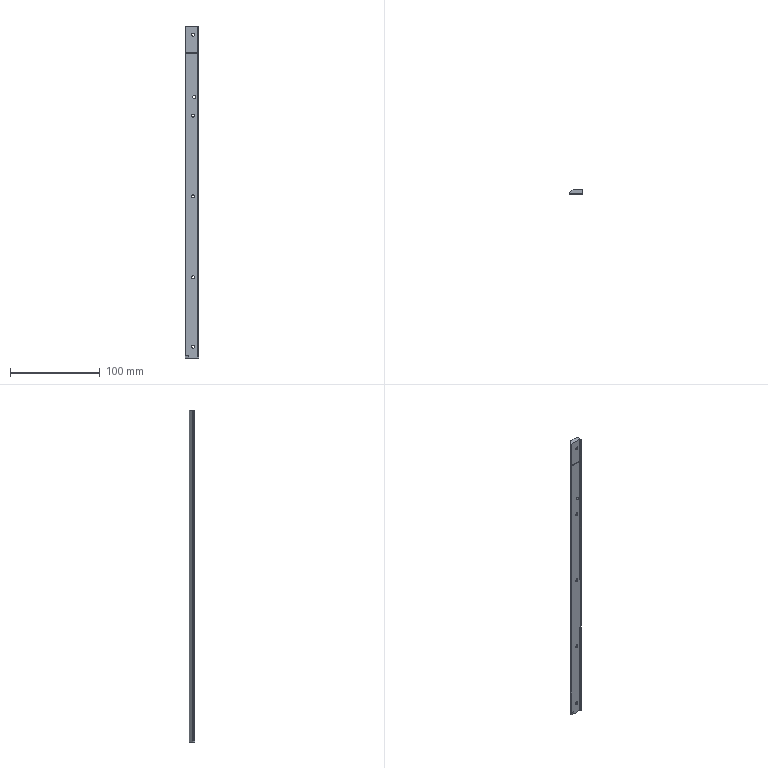Part | STEP file | 11-FG-B07611 | 1 solid | 45 faces | box 14.5 x 6 x 369.8 mm | volume 23525 mm3 | cylinder 23 | plane 22 | commonest cylinder face diameters 3.4 x10 6.5 x10 3.3 x2 0.85 x1
STEP:
#1=CARTESIAN_POINT('',(9.5,0.,289.15));
#2=VERTEX_POINT('',#1);
#3=CARTESIAN_POINT('',(9.5,0.,292.45));
#4=VERTEX_POINT('',#3);
#5=CARTESIAN_POINT('',(9.5,0.,290.8));
#6=DIRECTION('',(0.,1.,0.));
#7=DIRECTION('',(0.,0.,1.));
#8=AXIS2_PLACEMENT_3D('',#5,#6,#7);
#9=CIRCLE('',#8,1.65);
#10=EDGE_CURVE('',#2,#4,#9,.T.);
#11=ORIENTED_EDGE('',*,*,#10,.F.);
#12=CARTESIAN_POINT('',(9.5,5.,289.15));
#13=VERTEX_POINT('',#12);
#14=CARTESIAN_POINT('',(9.5,5.,289.15));
#15=DIRECTION('',(0.,1.,0.));
#16=VECTOR('',#15,1000.);
#17=LINE('',#14,#16);
#18=EDGE_CURVE('',#2,#13,#17,.T.);
#19=ORIENTED_EDGE('',*,*,#18,.T.);
#20=CARTESIAN_POINT('',(9.5,5.,292.45));
#21=VERTEX_POINT('',#20);
#22=CARTESIAN_POINT('',(9.5,5.,290.8));
#23=DIRECTION('',(0.,1.,0.));
#24=DIRECTION('',(0.,0.,1.));
#25=AXIS2_PLACEMENT_3D('',#22,#23,#24);
#26=CIRCLE('',#25,1.65);
#27=EDGE_CURVE('',#13,#21,#26,.T.);
#28=ORIENTED_EDGE('',*,*,#27,.T.);
#29=CARTESIAN_POINT('',(9.5,5.,292.45));
#30=DIRECTION('',(0.,1.,0.));
#31=VECTOR('',#30,1000.);
#32=LINE('',#29,#31);
#33=EDGE_CURVE('',#4,#21,#32,.T.);
#34=ORIENTED_EDGE('',*,*,#33,.F.);
#35=EDGE_LOOP('',(#11,#19,#28,#34));
#36=FACE_OUTER_BOUND('',#35,.T.);
#37=CARTESIAN_POINT('',(9.5,5.,290.8));
#38=DIRECTION('',(0.,1.,0.));
#39=DIRECTION('',(0.,0.,1.));
#40=AXIS2_PLACEMENT_3D('',#37,#38,#39);
#41=CYLINDRICAL_SURFACE('',#40,1.65);
#42=ADVANCED_FACE('',(#36),#41,.F.);
#43=CARTESIAN_POINT('',(8.5,1.6,356.75));
#44=VERTEX_POINT('',#43);
#45=CARTESIAN_POINT('',(8.5,1.6,363.25));
#46=VERTEX_POINT('',#45);
#47=CARTESIAN_POINT('',(8.5,1.6,360.));
#48=DIRECTION('',(0.,1.,0.));
#49=DIRECTION('',(0.,0.,1.));
#50=AXIS2_PLACEMENT_3D('',#47,#48,#49);
#51=CIRCLE('',#50,3.25);
#52=EDGE_CURVE('',#44,#46,#51,.T.);
#53=ORIENTED_EDGE('',*,*,#52,.F.);
#54=CARTESIAN_POINT('',(8.5,5.,356.75));
#55=VERTEX_POINT('',#54);
#56=CARTESIAN_POINT('',(8.5,5.,356.75));
#57=DIRECTION('',(0.,1.,0.));
#58=VECTOR('',#57,1000.);
#59=LINE('',#56,#58);
#60=EDGE_CURVE('',#44,#55,#59,.T.);
#61=ORIENTED_EDGE('',*,*,#60,.T.);
#62=CARTESIAN_POINT('',(8.5,5.,363.25));
#63=VERTEX_POINT('',#62);
#64=CARTESIAN_POINT('',(8.5,5.,360.));
#65=DIRECTION('',(0.,1.,0.));
#66=DIRECTION('',(0.,0.,1.));
#67=AXIS2_PLACEMENT_3D('',#64,#65,#66);
#68=CIRCLE('',#67,3.25);
#69=EDGE_CURVE('',#55,#63,#68,.T.);
#70=ORIENTED_EDGE('',*,*,#69,.T.);
#71=CARTESIAN_POINT('',(8.5,5.,363.25));
#72=DIRECTION('',(0.,1.,0.));
#73=VECTOR('',#72,1000.);
#74=LINE('',#71,#73);
#75=EDGE_CURVE('',#46,#63,#74,.T.);
#76=ORIENTED_EDGE('',*,*,#75,.F.);
#77=EDGE_LOOP('',(#53,#61,#70,#76));
#78=FACE_OUTER_BOUND('',#77,.T.);
#79=CARTESIAN_POINT('',(8.5,5.,360.));
#80=DIRECTION('',(0.,1.,0.));
#81=DIRECTION('',(0.,0.,1.));
#82=AXIS2_PLACEMENT_3D('',#79,#80,#81);
#83=CYLINDRICAL_SURFACE('',#82,3.25);
#84=ADVANCED_FACE('',(#78),#83,.F.);
#85=CARTESIAN_POINT('',(8.5,0.,358.3));
#86=VERTEX_POINT('',#85);
#87=CARTESIAN_POINT('',(8.5,0.,361.7));
#88=VERTEX_POINT('',#87);
#89=CARTESIAN_POINT('',(8.5,0.,360.));
#90=DIRECTION('',(0.,1.,0.));
#91=DIRECTION('',(0.,0.,1.));
#92=AXIS2_PLACEMENT_3D('',#89,#90,#91);
#93=CIRCLE('',#92,1.7);
#94=EDGE_CURVE('',#86,#88,#93,.T.);
#95=ORIENTED_EDGE('',*,*,#94,.F.);
#96=CARTESIAN_POINT('',(8.5,1.6,358.3));
#97=VERTEX_POINT('',#96);
#98=CARTESIAN_POINT('',(8.5,5.,358.3));
#99=DIRECTION('',(0.,1.,0.));
#100=VECTOR('',#99,1000.);
#101=LINE('',#98,#100);
#102=EDGE_CURVE('',#86,#97,#101,.T.);
#103=ORIENTED_EDGE('',*,*,#102,.T.);
#104=CARTESIAN_POINT('',(8.5,1.6,361.7));
#105=VERTEX_POINT('',#104);
#106=CARTESIAN_POINT('',(8.5,1.6,360.));
#107=DIRECTION('',(0.,1.,0.));
#108=DIRECTION('',(0.,0.,1.));
#109=AXIS2_PLACEMENT_3D('',#106,#107,#108);
#110=CIRCLE('',#109,1.7);
#111=EDGE_CURVE('',#97,#105,#110,.T.);
#112=ORIENTED_EDGE('',*,*,#111,.T.);
#113=CARTESIAN_POINT('',(8.5,5.,361.7));
#114=DIRECTION('',(0.,1.,0.));
#115=VECTOR('',#114,1000.);
#116=LINE('',#113,#115);
#117=EDGE_CURVE('',#88,#105,#116,.T.);
#118=ORIENTED_EDGE('',*,*,#117,.F.);
#119=EDGE_LOOP('',(#95,#103,#112,#118));
#120=FACE_OUTER_BOUND('',#119,.T.);
#121=CARTESIAN_POINT('',(8.5,5.,360.));
#122=DIRECTION('',(0.,1.,0.));
#123=DIRECTION('',(0.,0.,1.));
#124=AXIS2_PLACEMENT_3D('',#121,#122,#123);
#125=CYLINDRICAL_SURFACE('',#124,1.7);
#126=ADVANCED_FACE('',(#120),#125,.F.);
#127=CARTESIAN_POINT('',(8.5,1.6,266.75));
#128=VERTEX_POINT('',#127);
#129=CARTESIAN_POINT('',(8.5,1.6,273.25));
#130=VERTEX_POINT('',#129);
#131=CARTESIAN_POINT('',(8.5,1.6,270.));
#132=DIRECTION('',(0.,1.,0.));
#133=DIRECTION('',(0.,0.,1.));
#134=AXIS2_PLACEMENT_3D('',#131,#132,#133);
#135=CIRCLE('',#134,3.25);
#136=EDGE_CURVE('',#128,#130,#135,.T.);
#137=ORIENTED_EDGE('',*,*,#136,.F.);
#138=CARTESIAN_POINT('',(8.5,5.,266.75));
#139=VERTEX_POINT('',#138);
#140=CARTESIAN_POINT('',(8.5,5.,266.75));
#141=DIRECTION('',(0.,1.,0.));
#142=VECTOR('',#141,1000.);
#143=LINE('',#140,#142);
#144=EDGE_CURVE('',#128,#139,#143,.T.);
#145=ORIENTED_EDGE('',*,*,#144,.T.);
#146=CARTESIAN_POINT('',(8.5,5.,273.25));
#147=VERTEX_POINT('',#146);
#148=CARTESIAN_POINT('',(8.5,5.,270.));
#149=DIRECTION('',(0.,1.,0.));
#150=DIRECTION('',(0.,0.,1.));
#151=AXIS2_PLACEMENT_3D('',#148,#149,#150);
#152=CIRCLE('',#151,3.25);
#153=EDGE_CURVE('',#139,#147,#152,.T.);
#154=ORIENTED_EDGE('',*,*,#153,.T.);
#155=CARTESIAN_POINT('',(8.5,5.,273.25));
#156=DIRECTION('',(0.,1.,0.));
#157=VECTOR('',#156,1000.);
#158=LINE('',#155,#157);
#159=EDGE_CURVE('',#130,#147,#158,.T.);
#160=ORIENTED_EDGE('',*,*,#159,.F.);
#161=EDGE_LOOP('',(#137,#145,#154,#160));
#162=FACE_OUTER_BOUND('',#161,.T.);
#163=CARTESIAN_POINT('',(8.5,5.,270.));
#164=DIRECTION('',(0.,1.,0.));
#165=DIRECTION('',(0.,0.,1.));
#166=AXIS2_PLACEMENT_3D('',#163,#164,#165);
#167=CYLINDRICAL_SURFACE('',#166,3.25);
#168=ADVANCED_FACE('',(#162),#167,.F.);
#169=CARTESIAN_POINT('',(8.5,0.,268.3));
#170=VERTEX_POINT('',#169);
#171=CARTESIAN_POINT('',(8.5,0.,271.7));
#172=VERTEX_POINT('',#171);
#173=CARTESIAN_POINT('',(8.5,0.,270.));
#174=DIRECTION('',(0.,1.,0.));
#175=DIRECTION('',(0.,0.,1.));
#176=AXIS2_PLACEMENT_3D('',#173,#174,#175);
#177=CIRCLE('',#176,1.7);
#178=EDGE_CURVE('',#170,#172,#177,.T.);
#179=ORIENTED_EDGE('',*,*,#178,.F.);
#180=CARTESIAN_POINT('',(8.5,1.6,268.3));
#181=VERTEX_POINT('',#180);
#182=CARTESIAN_POINT('',(8.5,5.,268.3));
#183=DIRECTION('',(0.,1.,0.));
#184=VECTOR('',#183,1000.);
#185=LINE('',#182,#184);
#186=EDGE_CURVE('',#170,#181,#185,.T.);
#187=ORIENTED_EDGE('',*,*,#186,.T.);
#188=CARTESIAN_POINT('',(8.5,1.6,271.7));
#189=VERTEX_POINT('',#188);
#190=CARTESIAN_POINT('',(8.5,1.6,270.));
#191=DIRECTION('',(0.,1.,0.));
#192=DIRECTION('',(0.,0.,1.));
#193=AXIS2_PLACEMENT_3D('',#190,#191,#192);
#194=CIRCLE('',#193,1.7);
#195=EDGE_CURVE('',#181,#189,#194,.T.);
#196=ORIENTED_EDGE('',*,*,#195,.T.);
#197=CARTESIAN_POINT('',(8.5,5.,271.7));
#198=DIRECTION('',(0.,1.,0.));
#199=VECTOR('',#198,1000.);
#200=LINE('',#197,#199);
#201=EDGE_CURVE('',#172,#189,#200,.T.);
#202=ORIENTED_EDGE('',*,*,#201,.F.);
#203=EDGE_LOOP('',(#179,#187,#196,#202));
#204=FACE_OUTER_BOUND('',#203,.T.);
#205=CARTESIAN_POINT('',(8.5,5.,270.));
#206=DIRECTION('',(0.,1.,0.));
#207=DIRECTION('',(0.,0.,1.));
#208=AXIS2_PLACEMENT_3D('',#205,#206,#207);
#209=CYLINDRICAL_SURFACE('',#208,1.7);
#210=ADVANCED_FACE('',(#204),#209,.F.);
#211=CARTESIAN_POINT('',(8.5,1.6,176.75));
#212=VERTEX_POINT('',#211);
#213=CARTESIAN_POINT('',(8.5,1.6,183.25));
#214=VERTEX_POINT('',#213);
#215=CARTESIAN_POINT('',(8.5,1.6,180.));
#216=DIRECTION('',(0.,1.,0.));
#217=DIRECTION('',(0.,0.,1.));
#218=AXIS2_PLACEMENT_3D('',#215,#216,#217);
#219=CIRCLE('',#218,3.25);
#220=EDGE_CURVE('',#212,#214,#219,.T.);
#221=ORIENTED_EDGE('',*,*,#220,.F.);
#222=CARTESIAN_POINT('',(8.5,5.,176.75));
#223=VERTEX_POINT('',#222);
#224=CARTESIAN_POINT('',(8.5,5.,176.75));
#225=DIRECTION('',(0.,1.,0.));
#226=VECTOR('',#225,1000.);
#227=LINE('',#224,#226);
#228=EDGE_CURVE('',#212,#223,#227,.T.);
#229=ORIENTED_EDGE('',*,*,#228,.T.);
#230=CARTESIAN_POINT('',(8.5,5.,183.25));
#231=VERTEX_POINT('',#230);
#232=CARTESIAN_POINT('',(8.5,5.,180.));
#233=DIRECTION('',(0.,1.,0.));
#234=DIRECTION('',(0.,0.,1.));
#235=AXIS2_PLACEMENT_3D('',#232,#233,#234);
#236=CIRCLE('',#235,3.25);
#237=EDGE_CURVE('',#223,#231,#236,.T.);
#238=ORIENTED_EDGE('',*,*,#237,.T.);
#239=CARTESIAN_POINT('',(8.5,5.,183.25));
#240=DIRECTION('',(0.,1.,0.));
#241=VECTOR('',#240,1000.);
#242=LINE('',#239,#241);
#243=EDGE_CURVE('',#214,#231,#242,.T.);
#244=ORIENTED_EDGE('',*,*,#243,.F.);
#245=EDGE_LOOP('',(#221,#229,#238,#244));
#246=FACE_OUTER_BOUND('',#245,.T.);
#247=CARTESIAN_POINT('',(8.5,5.,180.));
#248=DIRECTION('',(0.,1.,0.));
#249=DIRECTION('',(0.,0.,1.));
#250=AXIS2_PLACEMENT_3D('',#247,#248,#249);
#251=CYLINDRICAL_SURFACE('',#250,3.25);
#252=ADVANCED_FACE('',(#246),#251,.F.);
#253=CARTESIAN_POINT('',(8.5,0.,178.3));
#254=VERTEX_POINT('',#253);
#255=CARTESIAN_POINT('',(8.5,0.,181.7));
#256=VERTEX_POINT('',#255);
#257=CARTESIAN_POINT('',(8.5,0.,180.));
#258=DIRECTION('',(0.,1.,0.));
#259=DIRECTION('',(0.,0.,1.));
#260=AXIS2_PLACEMENT_3D('',#257,#258,#259);
#261=CIRCLE('',#260,1.7);
#262=EDGE_CURVE('',#254,#256,#261,.T.);
#263=ORIENTED_EDGE('',*,*,#262,.F.);
#264=CARTESIAN_POINT('',(8.5,1.6,178.3));
#265=VERTEX_POINT('',#264);
#266=CARTESIAN_POINT('',(8.5,5.,178.3));
#267=DIRECTION('',(0.,1.,0.));
#268=VECTOR('',#267,1000.);
#269=LINE('',#266,#268);
#270=EDGE_CURVE('',#254,#265,#269,.T.);
#271=ORIENTED_EDGE('',*,*,#270,.T.);
#272=CARTESIAN_POINT('',(8.5,1.6,181.7));
#273=VERTEX_POINT('',#272);
#274=CARTESIAN_POINT('',(8.5,1.6,180.));
#275=DIRECTION('',(0.,1.,0.));
#276=DIRECTION('',(0.,0.,1.));
#277=AXIS2_PLACEMENT_3D('',#274,#275,#276);
#278=CIRCLE('',#277,1.7);
#279=EDGE_CURVE('',#265,#273,#278,.T.);
#280=ORIENTED_EDGE('',*,*,#279,.T.);
#281=CARTESIAN_POINT('',(8.5,5.,181.7));
#282=DIRECTION('',(0.,1.,0.));
#283=VECTOR('',#282,1000.);
#284=LINE('',#281,#283);
#285=EDGE_CURVE('',#256,#273,#284,.T.);
#286=ORIENTED_EDGE('',*,*,#285,.F.);
#287=EDGE_LOOP('',(#263,#271,#280,#286));
#288=FACE_OUTER_BOUND('',#287,.T.);
#289=CARTESIAN_POINT('',(8.5,5.,180.));
#290=DIRECTION('',(0.,1.,0.));
#291=DIRECTION('',(0.,0.,1.));
#292=AXIS2_PLACEMENT_3D('',#289,#290,#291);
#293=CYLINDRICAL_SURFACE('',#292,1.7);
#294=ADVANCED_FACE('',(#288),#293,.F.);
#295=CARTESIAN_POINT('',(8.5,1.6,86.75));
#296=VERTEX_POINT('',#295);
#297=CARTESIAN_POINT('',(8.5,1.6,93.25));
#298=VERTEX_POINT('',#297);
#299=CARTESIAN_POINT('',(8.5,1.6,90.));
#300=DIRECTION('',(0.,1.,0.));
#301=DIRECTION('',(0.,0.,1.));
#302=AXIS2_PLACEMENT_3D('',#299,#300,#301);
#303=CIRCLE('',#302,3.25);
#304=EDGE_CURVE('',#296,#298,#303,.T.);
#305=ORIENTED_EDGE('',*,*,#304,.F.);
#306=CARTESIAN_POINT('',(8.5,5.,86.75));
#307=VERTEX_POINT('',#306);
#308=CARTESIAN_POINT('',(8.5,5.,86.75));
#309=DIRECTION('',(0.,1.,0.));
#310=VECTOR('',#309,1000.);
#311=LINE('',#308,#310);
#312=EDGE_CURVE('',#296,#307,#311,.T.);
#313=ORIENTED_EDGE('',*,*,#312,.T.);
#314=CARTESIAN_POINT('',(8.5,5.,93.25));
#315=VERTEX_POINT('',#314);
#316=CARTESIAN_POINT('',(8.5,5.,90.));
#317=DIRECTION('',(0.,1.,0.));
#318=DIRECTION('',(0.,0.,1.));
#319=AXIS2_PLACEMENT_3D('',#316,#317,#318);
#320=CIRCLE('',#319,3.25);
#321=EDGE_CURVE('',#307,#315,#320,.T.);
#322=ORIENTED_EDGE('',*,*,#321,.T.);
#323=CARTESIAN_POINT('',(8.5,5.,93.25));
#324=DIRECTION('',(0.,1.,0.));
#325=VECTOR('',#324,1000.);
#326=LINE('',#323,#325);
#327=EDGE_CURVE('',#298,#315,#326,.T.);
#328=ORIENTED_EDGE('',*,*,#327,.F.);
#329=EDGE_LOOP('',(#305,#313,#322,#328));
#330=FACE_OUTER_BOUND('',#329,.T.);
#331=CARTESIAN_POINT('',(8.5,5.,90.));
#332=DIRECTION('',(0.,1.,0.));
#333=DIRECTION('',(0.,0.,1.));
#334=AXIS2_PLACEMENT_3D('',#331,#332,#333);
#335=CYLINDRICAL_SURFACE('',#334,3.25);
#336=ADVANCED_FACE('',(#330),#335,.F.);
#337=CARTESIAN_POINT('',(8.5,0.,88.3));
#338=VERTEX_POINT('',#337);
#339=CARTESIAN_POINT('',(8.5,0.,91.7));
#340=VERTEX_POINT('',#339);
#341=CARTESIAN_POINT('',(8.5,0.,90.));
#342=DIRECTION('',(0.,1.,0.));
#343=DIRECTION('',(0.,0.,1.));
#344=AXIS2_PLACEMENT_3D('',#341,#342,#343);
#345=CIRCLE('',#344,1.7);
#346=EDGE_CURVE('',#338,#340,#345,.T.);
#347=ORIENTED_EDGE('',*,*,#346,.F.);
#348=CARTESIAN_POINT('',(8.5,1.6,88.3));
#349=VERTEX_POINT('',#348);
#350=CARTESIAN_POINT('',(8.5,5.,88.3));
#351=DIRECTION('',(0.,1.,0.));
#352=VECTOR('',#351,1000.);
#353=LINE('',#350,#352);
#354=EDGE_CURVE('',#338,#349,#353,.T.);
#355=ORIENTED_EDGE('',*,*,#354,.T.);
#356=CARTESIAN_POINT('',(8.5,1.6,91.7));
#357=VERTEX_POINT('',#356);
#358=CARTESIAN_POINT('',(8.5,1.6,90.));
#359=DIRECTION('',(0.,1.,0.));
#360=DIRECTION('',(0.,0.,1.));
#361=AXIS2_PLACEMENT_3D('',#358,#359,#360);
#362=CIRCLE('',#361,1.7);
#363=EDGE_CURVE('',#349,#357,#362,.T.);
#364=ORIENTED_EDGE('',*,*,#363,.T.);
#365=CARTESIAN_POINT('',(8.5,5.,91.7));
#366=DIRECTION('',(0.,1.,0.));
#367=VECTOR('',#366,1000.);
#368=LINE('',#365,#367);
#369=EDGE_CURVE('',#340,#357,#368,.T.);
#370=ORIENTED_EDGE('',*,*,#369,.F.);
#371=EDGE_LOOP('',(#347,#355,#364,#370));
#372=FACE_OUTER_BOUND('',#371,.T.);
#373=CARTESIAN_POINT('',(8.5,5.,90.));
#374=DIRECTION('',(0.,1.,0.));
#375=DIRECTION('',(0.,0.,1.));
#376=AXIS2_PLACEMENT_3D('',#373,#374,#375);
#377=CYLINDRICAL_SURFACE('',#376,1.7);
#378=ADVANCED_FACE('',(#372),#377,.F.);
#379=CARTESIAN_POINT('',(8.5,1.6,9.25));
#380=VERTEX_POINT('',#379);
#381=CARTESIAN_POINT('',(8.5,1.6,15.75));
#382=VERTEX_POINT('',#381);
#383=CARTESIAN_POINT('',(8.5,1.6,12.5));
#384=DIRECTION('',(0.,1.,0.));
#385=DIRECTION('',(0.,0.,1.));
#386=AXIS2_PLACEMENT_3D('',#383,#384,#385);
#387=CIRCLE('',#386,3.25);
#388=EDGE_CURVE('',#380,#382,#387,.T.);
#389=ORIENTED_EDGE('',*,*,#388,.F.);
#390=CARTESIAN_POINT('',(8.5,5.,9.25));
#391=VERTEX_POINT('',#390);
#392=CARTESIAN_POINT('',(8.5,5.,9.25));
#393=DIRECTION('',(0.,1.,0.));
#394=VECTOR('',#393,1000.);
#395=LINE('',#392,#394);
#396=EDGE_CURVE('',#380,#391,#395,.T.);
#397=ORIENTED_EDGE('',*,*,#396,.T.);
#398=CARTESIAN_POINT('',(8.5,5.,15.75));
#399=VERTEX_POINT('',#398);
#400=CARTESIAN_POINT('',(8.5,5.,12.5));
#401=DIRECTION('',(0.,1.,0.));
#402=DIRECTION('',(0.,0.,1.));
#403=AXIS2_PLACEMENT_3D('',#400,#401,#402);
#404=CIRCLE('',#403,3.25);
#405=EDGE_CURVE('',#391,#399,#404,.T.);
#406=ORIENTED_EDGE('',*,*,#405,.T.);
#407=CARTESIAN_POINT('',(8.5,5.,15.75));
#408=DIRECTION('',(0.,1.,0.));
#409=VECTOR('',#408,1000.);
#410=LINE('',#407,#409);
#411=EDGE_CURVE('',#382,#399,#410,.T.);
#412=ORIENTED_EDGE('',*,*,#411,.F.);
#413=EDGE_LOOP('',(#389,#397,#406,#412));
#414=FACE_OUTER_BOUND('',#413,.T.);
#415=CARTESIAN_POINT('',(8.5,5.,12.5));
#416=DIRECTION('',(0.,1.,0.));
#417=DIRECTION('',(0.,0.,1.));
#418=AXIS2_PLACEMENT_3D('',#415,#416,#417);
#419=CYLINDRICAL_SURFACE('',#418,3.25);
#420=ADVANCED_FACE('',(#414),#419,.F.);
#421=CARTESIAN_POINT('',(8.5,0.,10.8));
#422=VERTEX_POINT('',#421);
#423=CARTESIAN_POINT('',(8.5,0.,14.2));
#424=VERTEX_POINT('',#423);
#425=CARTESIAN_POINT('',(8.5,0.,12.5));
#426=DIRECTION('',(0.,1.,0.));
#427=DIRECTION('',(0.,0.,1.));
#428=AXIS2_PLACEMENT_3D('',#425,#426,#427);
#429=CIRCLE('',#428,1.7);
#430=EDGE_CURVE('',#422,#424,#429,.T.);
#431=ORIENTED_EDGE('',*,*,#430,.F.);
#432=CARTESIAN_POINT('',(8.5,1.6,10.8));
#433=VERTEX_POINT('',#432);
#434=CARTESIAN_POINT('',(8.5,5.,10.8));
#435=DIRECTION('',(0.,1.,0.));
#436=VECTOR('',#435,1000.);
#437=LINE('',#434,#436);
#438=EDGE_CURVE('',#422,#433,#437,.T.);
#439=ORIENTED_EDGE('',*,*,#438,.T.);
#440=CARTESIAN_POINT('',(8.5,1.6,14.2));
#441=VERTEX_POINT('',#440);
#442=CARTESIAN_POINT('',(8.5,1.6,12.5));
#443=DIRECTION('',(0.,1.,0.));
#444=DIRECTION('',(0.,0.,1.));
#445=AXIS2_PLACEMENT_3D('',#442,#443,#444);
#446=CIRCLE('',#445,1.7);
#447=EDGE_CURVE('',#433,#441,#446,.T.);
#448=ORIENTED_EDGE('',*,*,#447,.T.);
#449=CARTESIAN_POINT('',(8.5,5.,14.2));
#450=DIRECTION('',(0.,1.,0.));
#451=VECTOR('',#450,1000.);
#452=LINE('',#449,#451);
#453=EDGE_CURVE('',#424,#441,#452,.T.);
#454=ORIENTED_EDGE('',*,*,#453,.F.);
#455=EDGE_LOOP('',(#431,#439,#448,#454));
#456=FACE_OUTER_BOUND('',#455,.T.);
#457=CARTESIAN_POINT('',(8.5,5.,12.5));
#458=DIRECTION('',(0.,1.,0.));
#459=DIRECTION('',(0.,0.,1.));
#460=AXIS2_PLACEMENT_3D('',#457,#458,#459);
#461=CYLINDRICAL_SURFACE('',#460,1.7);
#462=ADVANCED_FACE('',(#456),#461,.F.);
#463=CARTESIAN_POINT('',(0.,0.,369.8));
#464=VERTEX_POINT('',#463);
#465=CARTESIAN_POINT('',(0.,0.,340.425));
#466=VERTEX_POINT('',#465);
#467=CARTESIAN_POINT('',(0.,0.,370.));
#468=DIRECTION('',(0.,0.,-1.));
#469=VECTOR('',#468,1000.);
#470=LINE('',#467,#469);
#471=EDGE_CURVE('',#464,#466,#470,.T.);
#472=ORIENTED_EDGE('',*,*,#471,.F.);
#473=CARTESIAN_POINT('',(0.,1.,369.8));
#474=VERTEX_POINT('',#473);
#475=CARTESIAN_POINT('',(0.,-42.,369.8));
#476=DIRECTION('',(0.,1.,0.));
#477=VECTOR('',#476,1000.);
#478=LINE('',#475,#477);
#479=EDGE_CURVE('',#464,#474,#478,.T.);
#480=ORIENTED_EDGE('',*,*,#479,.T.);
#481=CARTESIAN_POINT('',(0.,1.,340.144));
#482=VERTEX_POINT('',#481);
#483=CARTESIAN_POINT('',(0.,1.,370.));
#484=DIRECTION('',(0.,0.,-1.));
#485=VECTOR('',#484,1000.);
#486=LINE('',#483,#485);
#487=EDGE_CURVE('',#474,#482,#486,.T.);
#488=ORIENTED_EDGE('',*,*,#487,.T.);
#489=CARTESIAN_POINT('',(0.,0.6,340.425));
#490=VERTEX_POINT('',#489);
#491=CARTESIAN_POINT('',(0.,0.6,340.));
#492=DIRECTION('',(-1.,0.,0.));
#493=DIRECTION('',(0.,0.,1.));
#494=AXIS2_PLACEMENT_3D('',#491,#492,#493);
#495=CIRCLE('',#494,0.425);
#496=EDGE_CURVE('',#490,#482,#495,.T.);
#497=ORIENTED_EDGE('',*,*,#496,.F.);
#498=CARTESIAN_POINT('',(0.,0.6,340.425));
#499=DIRECTION('',(0.,1.,0.));
#500=VECTOR('',#499,1000.);
#501=LINE('',#498,#500);
#502=EDGE_CURVE('',#466,#490,#501,.T.);
#503=ORIENTED_EDGE('',*,*,#502,.F.);
#504=EDGE_LOOP('',(#472,#480,#488,#497,#503));
#505=FACE_OUTER_BOUND('',#504,.T.);
#506=CARTESIAN_POINT('',(0.,0.,370.));
#507=DIRECTION('',(1.,0.,0.));
#508=DIRECTION('',(0.,1.,0.));
#509=AXIS2_PLACEMENT_3D('',#506,#507,#508);
#510=PLANE('',#509);
#511=ADVANCED_FACE('',(#505),#510,.F.);
#512=CARTESIAN_POINT('',(8.5,0.,360.));
#513=DIRECTION('',(0.,1.,0.));
#514=DIRECTION('',(0.,0.,1.));
#515=AXIS2_PLACEMENT_3D('',#512,#513,#514);
#516=CIRCLE('',#515,1.7);
#517=EDGE_CURVE('',#88,#86,#516,.T.);
#518=ORIENTED_EDGE('',*,*,#517,.T.);
#519=ORIENTED_EDGE('',*,*,#94,.T.);
#520=EDGE_LOOP('',(#518,#519));
#521=FACE_BOUND('',#520,.T.);
#522=CARTESIAN_POINT('',(13.5,0.,369.8));
#523=VERTEX_POINT('',#522);
#524=CARTESIAN_POINT('',(13.5,0.,340.425));
#525=VERTEX_POINT('',#524);
#526=CARTESIAN_POINT('',(13.5,0.,370.));
#527=DIRECTION('',(0.,0.,-1.));
#528=VECTOR('',#527,1000.);
#529=LINE('',#526,#528);
#530=EDGE_CURVE('',#523,#525,#529,.T.);
#531=ORIENTED_EDGE('',*,*,#530,.F.);
#532=CARTESIAN_POINT('',(0.,0.,369.8));
#533=DIRECTION('',(-1.,0.,0.));
#534=VECTOR('',#533,1000.);
#535=LINE('',#532,#534);
#536=EDGE_CURVE('',#523,#464,#535,.T.);
#537=ORIENTED_EDGE('',*,*,#536,.T.);
#538=ORIENTED_EDGE('',*,*,#471,.T.);
#539=CARTESIAN_POINT('',(13.5,0.,340.425));
#540=DIRECTION('',(-1.,0.,0.));
#541=VECTOR('',#540,1000.);
#542=LINE('',#539,#541);
#543=EDGE_CURVE('',#525,#466,#542,.T.);
#544=ORIENTED_EDGE('',*,*,#543,.F.);
#545=EDGE_LOOP('',(#531,#537,#538,#544));
#546=FACE_OUTER_BOUND('',#545,.T.);
#547=CARTESIAN_POINT('',(0.,0.,370.));
#548=DIRECTION('',(0.,1.,0.));
#549=DIRECTION('',(0.,0.,1.));
#550=AXIS2_PLACEMENT_3D('',#547,#548,#549);
#551=PLANE('',#550);
#552=ADVANCED_FACE('',(#521,#546),#551,.F.);
#553=CARTESIAN_POINT('',(0.,1.,0.));
#554=VERTEX_POINT('',#553);
#555=CARTESIAN_POINT('',(0.,0.8038,0.));
#556=VERTEX_POINT('',#555);
#557=CARTESIAN_POINT('',(0.,0.,0.));
#558=DIRECTION('',(0.,-1.,0.));
#559=VECTOR('',#558,1000.);
#560=LINE('',#557,#559);
#561=EDGE_CURVE('',#554,#556,#560,.T.);
#562=ORIENTED_EDGE('',*,*,#561,.T.);
#563=CARTESIAN_POINT('',(0.,0.,3.));
#564=VERTEX_POINT('',#563);
#565=CARTESIAN_POINT('',(0.,0.,3.));
#566=DIRECTION('',(0.,0.2588,-0.9659));
#567=VECTOR('',#566,1000.);
#568=LINE('',#565,#567);
#569=EDGE_CURVE('',#564,#556,#568,.T.);
#570=ORIENTED_EDGE('',*,*,#569,.F.);
#571=CARTESIAN_POINT('',(0.,0.,339.575));
#572=VERTEX_POINT('',#571);
#573=CARTESIAN_POINT('',(0.,0.,370.));
#574=DIRECTION('',(0.,0.,-1.));
#575=VECTOR('',#574,1000.);
#576=LINE('',#573,#575);
#577=EDGE_CURVE('',#572,#564,#576,.T.);
#578=ORIENTED_EDGE('',*,*,#577,.F.);
#579=CARTESIAN_POINT('',(0.,0.6,339.575));
#580=VERTEX_POINT('',#579);
#581=CARTESIAN_POINT('',(0.,0.6,339.575));
#582=DIRECTION('',(0.,-1.,0.));
#583=VECTOR('',#582,1000.);
#584=LINE('',#581,#583);
#585=EDGE_CURVE('',#580,#572,#584,.T.);
#586=ORIENTED_EDGE('',*,*,#585,.F.);
#587=CARTESIAN_POINT('',(0.,1.,339.856));
#588=VERTEX_POINT('',#587);
#589=CARTESIAN_POINT('',(0.,0.6,340.));
#590=DIRECTION('',(-1.,0.,0.));
#591=DIRECTION('',(0.,0.,1.));
#592=AXIS2_PLACEMENT_3D('',#589,#590,#591);
#593=CIRCLE('',#592,0.425);
#594=EDGE_CURVE('',#588,#580,#593,.T.);
#595=ORIENTED_EDGE('',*,*,#594,.F.);
#596=CARTESIAN_POINT('',(0.,1.,370.));
#597=DIRECTION('',(0.,0.,-1.));
#598=VECTOR('',#597,1000.);
#599=LINE('',#596,#598);
#600=EDGE_CURVE('',#588,#554,#599,.T.);
#601=ORIENTED_EDGE('',*,*,#600,.T.);
#602=EDGE_LOOP('',(#562,#570,#578,#586,#595,#601));
#603=FACE_OUTER_BOUND('',#602,.T.);
#604=CARTESIAN_POINT('',(0.,0.,370.));
#605=DIRECTION('',(1.,0.,0.));
#606=DIRECTION('',(0.,1.,0.));
#607=AXIS2_PLACEMENT_3D('',#604,#605,#606);
#608=PLANE('',#607);
#609=ADVANCED_FACE('',(#603),#608,.F.);
#610=CARTESIAN_POINT('',(9.5,0.,290.8));
#611=DIRECTION('',(0.,1.,0.));
#612=DIRECTION('',(0.,0.,1.));
#613=AXIS2_PLACEMENT_3D('',#610,#611,#612);
#614=CIRCLE('',#613,1.65);
#615=EDGE_CURVE('',#4,#2,#614,.T.);
#616=ORIENTED_EDGE('',*,*,#615,.T.);
#617=ORIENTED_EDGE('',*,*,#10,.T.);
#618=EDGE_LOOP('',(#616,#617));
#619=FACE_BOUND('',#618,.T.);
#620=CARTESIAN_POINT('',(8.5,0.,270.));
#621=DIRECTION('',(0.,1.,0.));
#622=DIRECTION('',(0.,0.,1.));
#623=AXIS2_PLACEMENT_3D('',#620,#621,#622);
#624=CIRCLE('',#623,1.7);
#625=EDGE_CURVE('',#172,#170,#624,.T.);
#626=ORIENTED_EDGE('',*,*,#625,.T.);
#627=ORIENTED_EDGE('',*,*,#178,.T.);
#628=EDGE_LOOP('',(#626,#627));
#629=FACE_BOUND('',#628,.T.);
#630=CARTESIAN_POINT('',(8.5,0.,180.));
#631=DIRECTION('',(0.,1.,0.));
#632=DIRECTION('',(0.,0.,1.));
#633=AXIS2_PLACEMENT_3D('',#630,#631,#632);
#634=CIRCLE('',#633,1.7);
#635=EDGE_CURVE('',#256,#254,#634,.T.);
#636=ORIENTED_EDGE('',*,*,#635,.T.);
#637=ORIENTED_EDGE('',*,*,#262,.T.);
#638=EDGE_LOOP('',(#636,#637));
#639=FACE_BOUND('',#638,.T.);
#640=CARTESIAN_POINT('',(8.5,0.,90.));
#641=DIRECTION('',(0.,1.,0.));
#642=DIRECTION('',(0.,0.,1.));
#643=AXIS2_PLACEMENT_3D('',#640,#641,#642);
#644=CIRCLE('',#643,1.7);
#645=EDGE_CURVE('',#340,#338,#644,.T.);
#646=ORIENTED_EDGE('',*,*,#645,.T.);
#647=ORIENTED_EDGE('',*,*,#346,.T.);
#648=EDGE_LOOP('',(#646,#647));
#649=FACE_BOUND('',#648,.T.);
#650=CARTESIAN_POINT('',(8.5,0.,12.5));
#651=DIRECTION('',(0.,1.,0.));
#652=DIRECTION('',(0.,0.,1.));
#653=AXIS2_PLACEMENT_3D('',#650,#651,#652);
#654=CIRCLE('',#653,1.7);
#655=EDGE_CURVE('',#424,#422,#654,.T.);
#656=ORIENTED_EDGE('',*,*,#655,.T.);
#657=ORIENTED_EDGE('',*,*,#430,.T.);
#658=EDGE_LOOP('',(#656,#657));
#659=FACE_BOUND('',#658,.T.);
#660=CARTESIAN_POINT('',(3.5,0.,3.));
#661=VERTEX_POINT('',#660);
#662=CARTESIAN_POINT('',(3.5,0.,3.));
#663=DIRECTION('',(-1.,0.,0.));
#664=VECTOR('',#663,1000.);
#665=LINE('',#662,#664);
#666=EDGE_CURVE('',#661,#564,#665,.T.);
#667=ORIENTED_EDGE('',*,*,#666,.F.);
#668=CARTESIAN_POINT('',(4.304,0.,0.));
#669=VERTEX_POINT('',#668);
#670=CARTESIAN_POINT('',(3.5,0.,3.));
#671=DIRECTION('',(0.2588,0.,-0.9659));
#672=VECTOR('',#671,1000.);
#673=LINE('',#670,#672);
#674=EDGE_CURVE('',#661,#669,#673,.T.);
#675=ORIENTED_EDGE('',*,*,#674,.T.);
#676=CARTESIAN_POINT('',(13.5,0.,0.));
#677=VERTEX_POINT('',#676);
#678=CARTESIAN_POINT('',(0.,0.,0.));
#679=DIRECTION('',(1.,0.,0.));
#680=VECTOR('',#679,1000.);
#681=LINE('',#678,#680);
#682=EDGE_CURVE('',#669,#677,#681,.T.);
#683=ORIENTED_EDGE('',*,*,#682,.T.);
#684=CARTESIAN_POINT('',(13.5,0.,339.575));
#685=VERTEX_POINT('',#684);
#686=CARTESIAN_POINT('',(13.5,0.,370.));
#687=DIRECTION('',(0.,0.,-1.));
#688=VECTOR('',#687,1000.);
#689=LINE('',#686,#688);
#690=EDGE_CURVE('',#685,#677,#689,.T.);
#691=ORIENTED_EDGE('',*,*,#690,.F.);
#692=CARTESIAN_POINT('',(13.5,0.,339.575));
#693=DIRECTION('',(-1.,0.,0.));
#694=VECTOR('',#693,1000.);
#695=LINE('',#692,#694);
#696=EDGE_CURVE('',#685,#572,#695,.T.);
#697=ORIENTED_EDGE('',*,*,#696,.T.);
#698=ORIENTED_EDGE('',*,*,#577,.T.);
#699=EDGE_LOOP('',(#667,#675,#683,#691,#697,#698));
#700=FACE_OUTER_BOUND('',#699,.T.);
#701=CARTESIAN_POINT('',(0.,0.,370.));
#702=DIRECTION('',(0.,1.,0.));
#703=DIRECTION('',(0.,0.,1.));
#704=AXIS2_PLACEMENT_3D('',#701,#702,#703);
#705=PLANE('',#704);
#706=ADVANCED_FACE('',(#619,#629,#639,#649,#659,#700),#705,.F.);
#707=CARTESIAN_POINT('',(9.5,5.,290.8));
#708=DIRECTION('',(0.,1.,0.));
#709=DIRECTION('',(0.,0.,1.));
#710=AXIS2_PLACEMENT_3D('',#707,#708,#709);
#711=CIRCLE('',#710,1.65);
#712=EDGE_CURVE('',#21,#13,#711,.T.);
#713=ORIENTED_EDGE('',*,*,#712,.F.);
#714=ORIENTED_EDGE('',*,*,#27,.F.);
#715=EDGE_LOOP('',(#713,#714));
#716=FACE_BOUND('',#715,.T.);
#717=CARTESIAN_POINT('',(8.5,5.,360.));
#718=DIRECTION('',(0.,1.,0.));
#719=DIRECTION('',(0.,0.,1.));
#720=AXIS2_PLACEMENT_3D('',#717,#718,#719);
#721=CIRCLE('',#720,3.25);
#722=EDGE_CURVE('',#63,#55,#721,.T.);
#723=ORIENTED_EDGE('',*,*,#722,.F.);
#724=ORIENTED_EDGE('',*,*,#69,.F.);
#725=EDGE_LOOP('',(#723,#724));
#726=FACE_BOUND('',#725,.T.);
#727=CARTESIAN_POINT('',(8.5,5.,270.));
#728=DIRECTION('',(0.,1.,0.));
#729=DIRECTION('',(0.,0.,1.));
#730=AXIS2_PLACEMENT_3D('',#727,#728,#729);
#731=CIRCLE('',#730,3.25);
#732=EDGE_CURVE('',#147,#139,#731,.T.);
#733=ORIENTED_EDGE('',*,*,#732,.F.);
#734=ORIENTED_EDGE('',*,*,#153,.F.);
#735=EDGE_LOOP('',(#733,#734));
#736=FACE_BOUND('',#735,.T.);
#737=CARTESIAN_POINT('',(8.5,5.,180.));
#738=DIRECTION('',(0.,1.,0.));
#739=DIRECTION('',(0.,0.,1.));
#740=AXIS2_PLACEMENT_3D('',#737,#738,#739);
#741=CIRCLE('',#740,3.25);
#742=EDGE_CURVE('',#231,#223,#741,.T.);
#743=ORIENTED_EDGE('',*,*,#742,.F.);
#744=ORIENTED_EDGE('',*,*,#237,.F.);
#745=EDGE_LOOP('',(#743,#744));
#746=FACE_BOUND('',#745,.T.);
#747=CARTESIAN_POINT('',(8.5,5.,90.));
#748=DIRECTION('',(0.,1.,0.));
#749=DIRECTION('',(0.,0.,1.));
#750=AXIS2_PLACEMENT_3D('',#747,#748,#749);
#751=CIRCLE('',#750,3.25);
#752=EDGE_CURVE('',#315,#307,#751,.T.);
#753=ORIENTED_EDGE('',*,*,#752,.F.);
#754=ORIENTED_EDGE('',*,*,#321,.F.);
#755=EDGE_LOOP('',(#753,#754));
#756=FACE_BOUND('',#755,.T.);
#757=CARTESIAN_POINT('',(8.5,5.,12.5));
#758=DIRECTION('',(0.,1.,0.));
#759=DIRECTION('',(0.,0.,1.));
#760=AXIS2_PLACEMENT_3D('',#757,#758,#759);
#761=CIRCLE('',#760,3.25);
#762=EDGE_CURVE('',#399,#391,#761,.T.);
#763=ORIENTED_EDGE('',*,*,#762,.F.);
#764=ORIENTED_EDGE('',*,*,#405,.F.);
#765=EDGE_LOOP('',(#763,#764));
#766=FACE_BOUND('',#765,.T.);
#767=CARTESIAN_POINT('',(4.,5.,0.));
#768=VERTEX_POINT('',#767);
#769=CARTESIAN_POINT('',(4.,5.,369.8));
#770=VERTEX_POINT('',#769);
#771=CARTESIAN_POINT('',(4.,5.,370.));
#772=DIRECTION('',(0.,0.,1.));
#773=VECTOR('',#772,1000.);
#774=LINE('',#771,#773);
#775=EDGE_CURVE('',#768,#770,#774,.T.);
#776=ORIENTED_EDGE('',*,*,#775,.T.);
#777=CARTESIAN_POINT('',(14.5,5.,369.8));
#778=VERTEX_POINT('',#777);
#779=CARTESIAN_POINT('',(14.5,5.,369.8));
#780=DIRECTION('',(-1.,0.,0.));
#781=VECTOR('',#780,1000.);
#782=LINE('',#779,#781);
#783=EDGE_CURVE('',#778,#770,#782,.T.);
#784=ORIENTED_EDGE('',*,*,#783,.F.);
#785=CARTESIAN_POINT('',(14.5,5.,0.));
#786=VERTEX_POINT('',#785);
#787=CARTESIAN_POINT('',(14.5,5.,370.));
#788=DIRECTION('',(0.,0.,1.));
#789=VECTOR('',#788,1000.);
#790=LINE('',#787,#789);
#791=EDGE_CURVE('',#786,#778,#790,.T.);
#792=ORIENTED_EDGE('',*,*,#791,.F.);
#793=CARTESIAN_POINT('',(0.,5.,0.));
#794=DIRECTION('',(-1.,0.,0.));
#795=VECTOR('',#794,1000.);
#796=LINE('',#793,#795);
#797=EDGE_CURVE('',#786,#768,#796,.T.);
#798=ORIENTED_EDGE('',*,*,#797,.T.);
#799=EDGE_LOOP('',(#776,#784,#792,#798));
#800=FACE_OUTER_BOUND('',#799,.T.);
#801=CARTESIAN_POINT('',(0.,5.,370.));
#802=DIRECTION('',(0.,-1.,0.));
#803=DIRECTION('',(0.,0.,-1.));
#804=AXIS2_PLACEMENT_3D('',#801,#802,#803);
#805=PLANE('',#804);
#806=ADVANCED_FACE('',(#716,#726,#736,#746,#756,#766,#800),#805,.F.);
#807=ORIENTED_EDGE('',*,*,#682,.F.);
#808=CARTESIAN_POINT('',(4.304,0.8038,0.));
#809=VERTEX_POINT('',#808);
#810=CARTESIAN_POINT('',(4.304,0.8038,0.));
#811=DIRECTION('',(0.,1.,0.));
#812=VECTOR('',#811,1000.);
#813=LINE('',#810,#812);
#814=EDGE_CURVE('',#669,#809,#813,.T.);
#815=ORIENTED_EDGE('',*,*,#814,.T.);
#816=CARTESIAN_POINT('',(3.5,0.8038,0.));
#817=DIRECTION('',(-1.,0.,0.));
#818=VECTOR('',#817,1000.);
#819=LINE('',#816,#818);
#820=EDGE_CURVE('',#809,#556,#819,.T.);
#821=ORIENTED_EDGE('',*,*,#820,.T.);
#822=ORIENTED_EDGE('',*,*,#561,.F.);
#823=CARTESIAN_POINT('',(2.,3.,0.));
#824=DIRECTION('',(0.7071,0.7071,0.));
#825=VECTOR('',#824,1000.);
#826=LINE('',#823,#825);
#827=EDGE_CURVE('',#554,#768,#826,.T.);
#828=ORIENTED_EDGE('',*,*,#827,.T.);
#829=ORIENTED_EDGE('',*,*,#797,.F.);
#830=CARTESIAN_POINT('',(14.5,-1.,0.));
#831=VERTEX_POINT('',#830);
#832=CARTESIAN_POINT('',(14.5,5.,0.));
#833=DIRECTION('',(0.,1.,0.));
#834=VECTOR('',#833,1000.);
#835=LINE('',#832,#834);
#836=EDGE_CURVE('',#831,#786,#835,.T.);
#837=ORIENTED_EDGE('',*,*,#836,.F.);
#838=CARTESIAN_POINT('',(13.5,-1.,0.));
#839=VERTEX_POINT('',#838);
#840=CARTESIAN_POINT('',(14.5,-1.,0.));
#841=DIRECTION('',(-1.,0.,0.));
#842=VECTOR('',#841,1000.);
#843=LINE('',#840,#842);
#844=EDGE_CURVE('',#831,#839,#843,.T.);
#845=ORIENTED_EDGE('',*,*,#844,.T.);
#846=CARTESIAN_POINT('',(13.5,5.,0.));
#847=DIRECTION('',(0.,1.,0.));
#848=VECTOR('',#847,1000.);
#849=LINE('',#846,#848);
#850=EDGE_CURVE('',#839,#677,#849,.T.);
#851=ORIENTED_EDGE('',*,*,#850,.T.);
#852=EDGE_LOOP('',(#807,#815,#821,#822,#828,#829,#837,#845,#851));
#853=FACE_OUTER_BOUND('',#852,.T.);
#854=CARTESIAN_POINT('',(0.,5.,0.));
#855=DIRECTION('',(0.,0.,-1.));
#856=DIRECTION('',(-1.,0.,0.));
#857=AXIS2_PLACEMENT_3D('',#854,#855,#856);
#858=PLANE('',#857);
#859=ADVANCED_FACE('',(#853),#858,.T.);
#860=CARTESIAN_POINT('',(0.,1.,369.8));
#861=DIRECTION('',(-0.7071,-0.7071,0.));
#862=VECTOR('',#861,1000.);
#863=LINE('',#860,#862);
#864=EDGE_CURVE('',#770,#474,#863,.T.);
#865=ORIENTED_EDGE('',*,*,#864,.F.);
#866=ORIENTED_EDGE('',*,*,#775,.F.);
#867=ORIENTED_EDGE('',*,*,#827,.F.);
#868=ORIENTED_EDGE('',*,*,#600,.F.);
#869=CARTESIAN_POINT('',(0.,1.,340.144));
#870=CARTESIAN_POINT('',(0.03367,1.034,340.05));
#871=CARTESIAN_POINT('',(0.03367,1.034,339.95));
#872=CARTESIAN_POINT('',(0.,1.,339.856));
#873=(BOUNDED_CURVE()B_SPLINE_CURVE(3,(#869,#870,#871,#872),.UNSPECIFIED.,.F.,.F.)B_SPLINE_CURVE_WITH_KNOTS((4,4),(2.797,3.486),.UNSPECIFIED.)CURVE()GEOMETRIC_REPRESENTATION_ITEM()RATIONAL_B_SPLINE_CURVE((1.,0.9608,0.9608,1.))REPRESENTATION_ITEM(''));
#874=EDGE_CURVE('',#482,#588,#873,.T.);
#875=ORIENTED_EDGE('',*,*,#874,.F.);
#876=ORIENTED_EDGE('',*,*,#487,.F.);
#877=EDGE_LOOP('',(#865,#866,#867,#868,#875,#876));
#878=FACE_OUTER_BOUND('',#877,.T.);
#879=CARTESIAN_POINT('',(0.,1.,370.));
#880=DIRECTION('',(0.7071,-0.7071,0.));
#881=DIRECTION('',(0.7071,0.7071,0.));
#882=AXIS2_PLACEMENT_3D('',#879,#880,#881);
#883=PLANE('',#882);
#884=ADVANCED_FACE('',(#878),#883,.F.);
#885=ORIENTED_EDGE('',*,*,#874,.T.);
#886=ORIENTED_EDGE('',*,*,#594,.T.);
#887=CARTESIAN_POINT('',(14.5,0.6,339.575));
#888=VERTEX_POINT('',#887);
#889=CARTESIAN_POINT('',(13.5,0.6,339.575));
#890=DIRECTION('',(-1.,0.,0.));
#891=VECTOR('',#890,1000.);
#892=LINE('',#889,#891);
#893=EDGE_CURVE('',#888,#580,#892,.T.);
#894=ORIENTED_EDGE('',*,*,#893,.F.);
#895=CARTESIAN_POINT('',(14.5,0.6,340.425));
#896=VERTEX_POINT('',#895);
#897=CARTESIAN_POINT('',(14.5,0.6,340.));
#898=DIRECTION('',(-1.,0.,0.));
#899=DIRECTION('',(0.,1.,0.));
#900=AXIS2_PLACEMENT_3D('',#897,#898,#899);
#901=CIRCLE('',#900,0.425);
#902=EDGE_CURVE('',#896,#888,#901,.T.);
#903=ORIENTED_EDGE('',*,*,#902,.F.);
#904=CARTESIAN_POINT('',(13.5,0.6,340.425));
#905=DIRECTION('',(-1.,0.,0.));
#906=VECTOR('',#905,1000.);
#907=LINE('',#904,#906);
#908=EDGE_CURVE('',#896,#490,#907,.T.);
#909=ORIENTED_EDGE('',*,*,#908,.T.);
#910=ORIENTED_EDGE('',*,*,#496,.T.);
#911=EDGE_LOOP('',(#885,#886,#894,#903,#909,#910));
#912=FACE_OUTER_BOUND('',#911,.T.);
#913=CARTESIAN_POINT('',(13.5,0.6,340.));
#914=DIRECTION('',(-1.,0.,0.));
#915=DIRECTION('',(0.,0.,1.));
#916=AXIS2_PLACEMENT_3D('',#913,#914,#915);
#917=CYLINDRICAL_SURFACE('',#916,0.425);
#918=ADVANCED_FACE('',(#912),#917,.F.);
#919=ORIENTED_EDGE('',*,*,#502,.T.);
#920=ORIENTED_EDGE('',*,*,#908,.F.);
#921=CARTESIAN_POINT('',(14.5,-1.,340.425));
#922=VERTEX_POINT('',#921);
#923=CARTESIAN_POINT('',(14.5,0.6,340.425));
#924=DIRECTION('',(0.,1.,0.));
#925=VECTOR('',#924,1000.);
#926=LINE('',#923,#925);
#927=EDGE_CURVE('',#922,#896,#926,.T.);
#928=ORIENTED_EDGE('',*,*,#927,.F.);
#929=CARTESIAN_POINT('',(13.5,-1.,340.425));
#930=VERTEX_POINT('',#929);
#931=CARTESIAN_POINT('',(14.5,-1.,340.425));
#932=DIRECTION('',(-1.,0.,0.));
#933=VECTOR('',#932,1000.);
#934=LINE('',#931,#933);
#935=EDGE_CURVE('',#922,#930,#934,.T.);
#936=ORIENTED_EDGE('',*,*,#935,.T.);
#937=CARTESIAN_POINT('',(13.5,0.6,340.425));
#938=DIRECTION('',(0.,1.,0.));
#939=VECTOR('',#938,1000.);
#940=LINE('',#937,#939);
#941=EDGE_CURVE('',#930,#525,#940,.T.);
#942=ORIENTED_EDGE('',*,*,#941,.T.);
#943=ORIENTED_EDGE('',*,*,#543,.T.);
#944=EDGE_LOOP('',(#919,#920,#928,#936,#942,#943));
#945=FACE_OUTER_BOUND('',#944,.T.);
#946=CARTESIAN_POINT('',(13.5,0.6,340.425));
#947=DIRECTION('',(0.,0.,1.));
#948=DIRECTION('',(1.,0.,0.));
#949=AXIS2_PLACEMENT_3D('',#946,#947,#948);
#950=PLANE('',#949);
#951=ADVANCED_FACE('',(#945),#950,.F.);
#952=ORIENTED_EDGE('',*,*,#585,.T.);
#953=ORIENTED_EDGE('',*,*,#696,.F.);
#954=CARTESIAN_POINT('',(13.5,-1.,339.575));
#955=VERTEX_POINT('',#954);
#956=CARTESIAN_POINT('',(13.5,0.6,339.575));
#957=DIRECTION('',(0.,-1.,0.));
#958=VECTOR('',#957,1000.);
#959=LINE('',#956,#958);
#960=EDGE_CURVE('',#685,#955,#959,.T.);
#961=ORIENTED_EDGE('',*,*,#960,.T.);
#962=CARTESIAN_POINT('',(14.5,-1.,339.575));
#963=VERTEX_POINT('',#962);
#964=CARTESIAN_POINT('',(14.5,-1.,339.575));
#965=DIRECTION('',(-1.,0.,0.));
#966=VECTOR('',#965,1000.);
#967=LINE('',#964,#966);
#968=EDGE_CURVE('',#963,#955,#967,.T.);
#969=ORIENTED_EDGE('',*,*,#968,.F.);
#970=CARTESIAN_POINT('',(14.5,0.6,339.575));
#971=DIRECTION('',(0.,-1.,0.));
#972=VECTOR('',#971,1000.);
#973=LINE('',#970,#972);
#974=EDGE_CURVE('',#888,#963,#973,.T.);
#975=ORIENTED_EDGE('',*,*,#974,.F.);
#976=ORIENTED_EDGE('',*,*,#893,.T.);
#977=EDGE_LOOP('',(#952,#953,#961,#969,#975,#976));
#978=FACE_OUTER_BOUND('',#977,.T.);
#979=CARTESIAN_POINT('',(13.5,0.6,339.575));
#980=DIRECTION('',(0.,0.,-1.));
#981=DIRECTION('',(-1.,0.,0.));
#982=AXIS2_PLACEMENT_3D('',#979,#980,#981);
#983=PLANE('',#982);
#984=ADVANCED_FACE('',(#978),#983,.F.);
#985=ORIENTED_EDGE('',*,*,#438,.F.);
#986=ORIENTED_EDGE('',*,*,#655,.F.);
#987=ORIENTED_EDGE('',*,*,#453,.T.);
#988=CARTESIAN_POINT('',(8.5,1.6,12.5));
#989=DIRECTION('',(0.,1.,0.));
#990=DIRECTION('',(0.,0.,1.));
#991=AXIS2_PLACEMENT_3D('',#988,#989,#990);
#992=CIRCLE('',#991,1.7);
#993=EDGE_CURVE('',#441,#433,#992,.T.);
#994=ORIENTED_EDGE('',*,*,#993,.T.);
#995=EDGE_LOOP('',(#985,#986,#987,#994));
#996=FACE_OUTER_BOUND('',#995,.T.);
#997=CARTESIAN_POINT('',(8.5,5.,12.5));
#998=DIRECTION('',(0.,1.,0.));
#999=DIRECTION('',(0.,0.,1.));
#1000=AXIS2_PLACEMENT_3D('',#997,#998,#999);
#1001=CYLINDRICAL_SURFACE('',#1000,1.7);
#1002=ADVANCED_FACE('',(#996),#1001,.F.);
#1003=ORIENTED_EDGE('',*,*,#993,.F.);
#1004=ORIENTED_EDGE('',*,*,#447,.F.);
#1005=EDGE_LOOP('',(#1003,#1004));
#1006=FACE_BOUND('',#1005,.T.);
#1007=CARTESIAN_POINT('',(8.5,1.6,12.5));
#1008=DIRECTION('',(0.,1.,0.));
#1009=DIRECTION('',(0.,0.,1.));
#1010=AXIS2_PLACEMENT_3D('',#1007,#1008,#1009);
#1011=CIRCLE('',#1010,3.25);
#1012=EDGE_CURVE('',#382,#380,#1011,.T.);
#1013=ORIENTED_EDGE('',*,*,#1012,.T.);
#1014=ORIENTED_EDGE('',*,*,#388,.T.);
#1015=EDGE_LOOP('',(#1013,#1014));
#1016=FACE_OUTER_BOUND('',#1015,.T.);
#1017=CARTESIAN_POINT('',(10.2,1.6,12.5));
#1018=DIRECTION('',(0.,-1.,0.));
#1019=DIRECTION('',(0.,0.,-1.));
#1020=AXIS2_PLACEMENT_3D('',#1017,#1018,#1019);
#1021=PLANE('',#1020);
#1022=ADVANCED_FACE('',(#1006,#1016),#1021,.F.);
#1023=ORIENTED_EDGE('',*,*,#396,.F.);
#1024=ORIENTED_EDGE('',*,*,#1012,.F.);
#1025=ORIENTED_EDGE('',*,*,#411,.T.);
#1026=ORIENTED_EDGE('',*,*,#762,.T.);
#1027=EDGE_LOOP('',(#1023,#1024,#1025,#1026));
#1028=FACE_OUTER_BOUND('',#1027,.T.);
#1029=CARTESIAN_POINT('',(8.5,5.,12.5));
#1030=DIRECTION('',(0.,1.,0.));
#1031=DIRECTION('',(0.,0.,1.));
#1032=AXIS2_PLACEMENT_3D('',#1029,#1030,#1031);
#1033=CYLINDRICAL_SURFACE('',#1032,3.25);
#1034=ADVANCED_FACE('',(#1028),#1033,.F.);
#1035=ORIENTED_EDGE('',*,*,#354,.F.);
#1036=ORIENTED_EDGE('',*,*,#645,.F.);
#1037=ORIENTED_EDGE('',*,*,#369,.T.);
#1038=CARTESIAN_POINT('',(8.5,1.6,90.));
#1039=DIRECTION('',(0.,1.,0.));
#1040=DIRECTION('',(0.,0.,1.));
#1041=AXIS2_PLACEMENT_3D('',#1038,#1039,#1040);
#1042=CIRCLE('',#1041,1.7);
#1043=EDGE_CURVE('',#357,#349,#1042,.T.);
#1044=ORIENTED_EDGE('',*,*,#1043,.T.);
#1045=EDGE_LOOP('',(#1035,#1036,#1037,#1044));
#1046=FACE_OUTER_BOUND('',#1045,.T.);
#1047=CARTESIAN_POINT('',(8.5,5.,90.));
#1048=DIRECTION('',(0.,1.,0.));
#1049=DIRECTION('',(0.,0.,1.));
#1050=AXIS2_PLACEMENT_3D('',#1047,#1048,#1049);
#1051=CYLINDRICAL_SURFACE('',#1050,1.7);
#1052=ADVANCED_FACE('',(#1046),#1051,.F.);
#1053=ORIENTED_EDGE('',*,*,#1043,.F.);
#1054=ORIENTED_EDGE('',*,*,#363,.F.);
#1055=EDGE_LOOP('',(#1053,#1054));
#1056=FACE_BOUND('',#1055,.T.);
#1057=CARTESIAN_POINT('',(8.5,1.6,90.));
#1058=DIRECTION('',(0.,1.,0.));
#1059=DIRECTION('',(0.,0.,1.));
#1060=AXIS2_PLACEMENT_3D('',#1057,#1058,#1059);
#1061=CIRCLE('',#1060,3.25);
#1062=EDGE_CURVE('',#298,#296,#1061,.T.);
#1063=ORIENTED_EDGE('',*,*,#1062,.T.);
#1064=ORIENTED_EDGE('',*,*,#304,.T.);
#1065=EDGE_LOOP('',(#1063,#1064));
#1066=FACE_OUTER_BOUND('',#1065,.T.);
#1067=CARTESIAN_POINT('',(10.2,1.6,90.));
#1068=DIRECTION('',(0.,-1.,0.));
#1069=DIRECTION('',(0.,0.,-1.));
#1070=AXIS2_PLACEMENT_3D('',#1067,#1068,#1069);
#1071=PLANE('',#1070);
#1072=ADVANCED_FACE('',(#1056,#1066),#1071,.F.);
#1073=ORIENTED_EDGE('',*,*,#312,.F.);
#1074=ORIENTED_EDGE('',*,*,#1062,.F.);
#1075=ORIENTED_EDGE('',*,*,#327,.T.);
#1076=ORIENTED_EDGE('',*,*,#752,.T.);
#1077=EDGE_LOOP('',(#1073,#1074,#1075,#1076));
#1078=FACE_OUTER_BOUND('',#1077,.T.);
#1079=CARTESIAN_POINT('',(8.5,5.,90.));
#1080=DIRECTION('',(0.,1.,0.));
#1081=DIRECTION('',(0.,0.,1.));
#1082=AXIS2_PLACEMENT_3D('',#1079,#1080,#1081);
#1083=CYLINDRICAL_SURFACE('',#1082,3.25);
#1084=ADVANCED_FACE('',(#1078),#1083,.F.);
#1085=ORIENTED_EDGE('',*,*,#270,.F.);
#1086=ORIENTED_EDGE('',*,*,#635,.F.);
#1087=ORIENTED_EDGE('',*,*,#285,.T.);
#1088=CARTESIAN_POINT('',(8.5,1.6,180.));
#1089=DIRECTION('',(0.,1.,0.));
#1090=DIRECTION('',(0.,0.,1.));
#1091=AXIS2_PLACEMENT_3D('',#1088,#1089,#1090);
#1092=CIRCLE('',#1091,1.7);
#1093=EDGE_CURVE('',#273,#265,#1092,.T.);
#1094=ORIENTED_EDGE('',*,*,#1093,.T.);
#1095=EDGE_LOOP('',(#1085,#1086,#1087,#1094));
#1096=FACE_OUTER_BOUND('',#1095,.T.);
#1097=CARTESIAN_POINT('',(8.5,5.,180.));
#1098=DIRECTION('',(0.,1.,0.));
#1099=DIRECTION('',(0.,0.,1.));
#1100=AXIS2_PLACEMENT_3D('',#1097,#1098,#1099);
#1101=CYLINDRICAL_SURFACE('',#1100,1.7);
#1102=ADVANCED_FACE('',(#1096),#1101,.F.);
#1103=ORIENTED_EDGE('',*,*,#1093,.F.);
#1104=ORIENTED_EDGE('',*,*,#279,.F.);
#1105=EDGE_LOOP('',(#1103,#1104));
#1106=FACE_BOUND('',#1105,.T.);
#1107=CARTESIAN_POINT('',(8.5,1.6,180.));
#1108=DIRECTION('',(0.,1.,0.));
#1109=DIRECTION('',(0.,0.,1.));
#1110=AXIS2_PLACEMENT_3D('',#1107,#1108,#1109);
#1111=CIRCLE('',#1110,3.25);
#1112=EDGE_CURVE('',#214,#212,#1111,.T.);
#1113=ORIENTED_EDGE('',*,*,#1112,.T.);
#1114=ORIENTED_EDGE('',*,*,#220,.T.);
#1115=EDGE_LOOP('',(#1113,#1114));
#1116=FACE_OUTER_BOUND('',#1115,.T.);
#1117=CARTESIAN_POINT('',(10.2,1.6,180.));
#1118=DIRECTION('',(0.,-1.,0.));
#1119=DIRECTION('',(0.,0.,-1.));
#1120=AXIS2_PLACEMENT_3D('',#1117,#1118,#1119);
#1121=PLANE('',#1120);
#1122=ADVANCED_FACE('',(#1106,#1116),#1121,.F.);
#1123=ORIENTED_EDGE('',*,*,#228,.F.);
#1124=ORIENTED_EDGE('',*,*,#1112,.F.);
#1125=ORIENTED_EDGE('',*,*,#243,.T.);
#1126=ORIENTED_EDGE('',*,*,#742,.T.);
#1127=EDGE_LOOP('',(#1123,#1124,#1125,#1126));
#1128=FACE_OUTER_BOUND('',#1127,.T.);
#1129=CARTESIAN_POINT('',(8.5,5.,180.));
#1130=DIRECTION('',(0.,1.,0.));
#1131=DIRECTION('',(0.,0.,1.));
#1132=AXIS2_PLACEMENT_3D('',#1129,#1130,#1131);
#1133=CYLINDRICAL_SURFACE('',#1132,3.25);
#1134=ADVANCED_FACE('',(#1128),#1133,.F.);
#1135=ORIENTED_EDGE('',*,*,#186,.F.);
#1136=ORIENTED_EDGE('',*,*,#625,.F.);
#1137=ORIENTED_EDGE('',*,*,#201,.T.);
#1138=CARTESIAN_POINT('',(8.5,1.6,270.));
#1139=DIRECTION('',(0.,1.,0.));
#1140=DIRECTION('',(0.,0.,1.));
#1141=AXIS2_PLACEMENT_3D('',#1138,#1139,#1140);
#1142=CIRCLE('',#1141,1.7);
#1143=EDGE_CURVE('',#189,#181,#1142,.T.);
#1144=ORIENTED_EDGE('',*,*,#1143,.T.);
#1145=EDGE_LOOP('',(#1135,#1136,#1137,#1144));
#1146=FACE_OUTER_BOUND('',#1145,.T.);
#1147=CARTESIAN_POINT('',(8.5,5.,270.));
#1148=DIRECTION('',(0.,1.,0.));
#1149=DIRECTION('',(0.,0.,1.));
#1150=AXIS2_PLACEMENT_3D('',#1147,#1148,#1149);
#1151=CYLINDRICAL_SURFACE('',#1150,1.7);
#1152=ADVANCED_FACE('',(#1146),#1151,.F.);
#1153=ORIENTED_EDGE('',*,*,#1143,.F.);
#1154=ORIENTED_EDGE('',*,*,#195,.F.);
#1155=EDGE_LOOP('',(#1153,#1154));
#1156=FACE_BOUND('',#1155,.T.);
#1157=CARTESIAN_POINT('',(8.5,1.6,270.));
#1158=DIRECTION('',(0.,1.,0.));
#1159=DIRECTION('',(0.,0.,1.));
#1160=AXIS2_PLACEMENT_3D('',#1157,#1158,#1159);
#1161=CIRCLE('',#1160,3.25);
#1162=EDGE_CURVE('',#130,#128,#1161,.T.);
#1163=ORIENTED_EDGE('',*,*,#1162,.T.);
#1164=ORIENTED_EDGE('',*,*,#136,.T.);
#1165=EDGE_LOOP('',(#1163,#1164));
#1166=FACE_OUTER_BOUND('',#1165,.T.);
#1167=CARTESIAN_POINT('',(10.2,1.6,270.));
#1168=DIRECTION('',(0.,-1.,0.));
#1169=DIRECTION('',(0.,0.,-1.));
#1170=AXIS2_PLACEMENT_3D('',#1167,#1168,#1169);
#1171=PLANE('',#1170);
#1172=ADVANCED_FACE('',(#1156,#1166),#1171,.F.);
#1173=ORIENTED_EDGE('',*,*,#144,.F.);
#1174=ORIENTED_EDGE('',*,*,#1162,.F.);
#1175=ORIENTED_EDGE('',*,*,#159,.T.);
#1176=ORIENTED_EDGE('',*,*,#732,.T.);
#1177=EDGE_LOOP('',(#1173,#1174,#1175,#1176));
#1178=FACE_OUTER_BOUND('',#1177,.T.);
#1179=CARTESIAN_POINT('',(8.5,5.,270.));
#1180=DIRECTION('',(0.,1.,0.));
#1181=DIRECTION('',(0.,0.,1.));
#1182=AXIS2_PLACEMENT_3D('',#1179,#1180,#1181);
#1183=CYLINDRICAL_SURFACE('',#1182,3.25);
#1184=ADVANCED_FACE('',(#1178),#1183,.F.);
#1185=ORIENTED_EDGE('',*,*,#102,.F.);
#1186=ORIENTED_EDGE('',*,*,#517,.F.);
#1187=ORIENTED_EDGE('',*,*,#117,.T.);
#1188=CARTESIAN_POINT('',(8.5,1.6,360.));
#1189=DIRECTION('',(0.,1.,0.));
#1190=DIRECTION('',(0.,0.,1.));
#1191=AXIS2_PLACEMENT_3D('',#1188,#1189,#1190);
#1192=CIRCLE('',#1191,1.7);
#1193=EDGE_CURVE('',#105,#97,#1192,.T.);
#1194=ORIENTED_EDGE('',*,*,#1193,.T.);
#1195=EDGE_LOOP('',(#1185,#1186,#1187,#1194));
#1196=FACE_OUTER_BOUND('',#1195,.T.);
#1197=CARTESIAN_POINT('',(8.5,5.,360.));
#1198=DIRECTION('',(0.,1.,0.));
#1199=DIRECTION('',(0.,0.,1.));
#1200=AXIS2_PLACEMENT_3D('',#1197,#1198,#1199);
#1201=CYLINDRICAL_SURFACE('',#1200,1.7);
#1202=ADVANCED_FACE('',(#1196),#1201,.F.);
#1203=ORIENTED_EDGE('',*,*,#1193,.F.);
#1204=ORIENTED_EDGE('',*,*,#111,.F.);
#1205=EDGE_LOOP('',(#1203,#1204));
#1206=FACE_BOUND('',#1205,.T.);
#1207=CARTESIAN_POINT('',(8.5,1.6,360.));
#1208=DIRECTION('',(0.,1.,0.));
#1209=DIRECTION('',(0.,0.,1.));
#1210=AXIS2_PLACEMENT_3D('',#1207,#1208,#1209);
#1211=CIRCLE('',#1210,3.25);
#1212=EDGE_CURVE('',#46,#44,#1211,.T.);
#1213=ORIENTED_EDGE('',*,*,#1212,.T.);
#1214=ORIENTED_EDGE('',*,*,#52,.T.);
#1215=EDGE_LOOP('',(#1213,#1214));
#1216=FACE_OUTER_BOUND('',#1215,.T.);
#1217=CARTESIAN_POINT('',(10.2,1.6,360.));
#1218=DIRECTION('',(0.,-1.,0.));
#1219=DIRECTION('',(0.,0.,-1.));
#1220=AXIS2_PLACEMENT_3D('',#1217,#1218,#1219);
#1221=PLANE('',#1220);
#1222=ADVANCED_FACE('',(#1206,#1216),#1221,.F.);
#1223=ORIENTED_EDGE('',*,*,#60,.F.);
#1224=ORIENTED_EDGE('',*,*,#1212,.F.);
#1225=ORIENTED_EDGE('',*,*,#75,.T.);
#1226=ORIENTED_EDGE('',*,*,#722,.T.);
#1227=EDGE_LOOP('',(#1223,#1224,#1225,#1226));
#1228=FACE_OUTER_BOUND('',#1227,.T.);
#1229=CARTESIAN_POINT('',(8.5,5.,360.));
#1230=DIRECTION('',(0.,1.,0.));
#1231=DIRECTION('',(0.,0.,1.));
#1232=AXIS2_PLACEMENT_3D('',#1229,#1230,#1231);
#1233=CYLINDRICAL_SURFACE('',#1232,3.25);
#1234=ADVANCED_FACE('',(#1228),#1233,.F.);
#1235=ORIENTED_EDGE('',*,*,#569,.T.);
#1236=ORIENTED_EDGE('',*,*,#820,.F.);
#1237=CARTESIAN_POINT('',(3.5,0.,3.));
#1238=DIRECTION('',(-0.2506,-0.2506,0.9351));
#1239=VECTOR('',#1238,1000.);
#1240=LINE('',#1237,#1239);
#1241=EDGE_CURVE('',#809,#661,#1240,.T.);
#1242=ORIENTED_EDGE('',*,*,#1241,.T.);
#1243=ORIENTED_EDGE('',*,*,#666,.T.);
#1244=EDGE_LOOP('',(#1235,#1236,#1242,#1243));
#1245=FACE_OUTER_BOUND('',#1244,.T.);
#1246=CARTESIAN_POINT('',(3.5,0.,3.));
#1247=DIRECTION('',(0.,0.9659,0.2588));
#1248=DIRECTION('',(0.,-0.2588,0.9659));
#1249=AXIS2_PLACEMENT_3D('',#1246,#1247,#1248);
#1250=PLANE('',#1249);
#1251=ADVANCED_FACE('',(#1245),#1250,.F.);
#1252=ORIENTED_EDGE('',*,*,#1241,.F.);
#1253=ORIENTED_EDGE('',*,*,#814,.F.);
#1254=ORIENTED_EDGE('',*,*,#674,.F.);
#1255=EDGE_LOOP('',(#1252,#1253,#1254));
#1256=FACE_OUTER_BOUND('',#1255,.T.);
#1257=CARTESIAN_POINT('',(3.5,0.,3.));
#1258=DIRECTION('',(-0.9659,0.,-0.2588));
#1259=DIRECTION('',(0.,1.,0.));
#1260=AXIS2_PLACEMENT_3D('',#1257,#1258,#1259);
#1261=PLANE('',#1260);
#1262=ADVANCED_FACE('',(#1256),#1261,.T.);
#1263=CARTESIAN_POINT('',(13.5,-1.,369.8));
#1264=VERTEX_POINT('',#1263);
#1265=CARTESIAN_POINT('',(13.5,-1.,370.));
#1266=DIRECTION('',(0.,0.,-1.));
#1267=VECTOR('',#1266,1000.);
#1268=LINE('',#1265,#1267);
#1269=EDGE_CURVE('',#1264,#930,#1268,.T.);
#1270=ORIENTED_EDGE('',*,*,#1269,.F.);
#1271=CARTESIAN_POINT('',(13.5,0.6,369.8));
#1272=DIRECTION('',(0.,1.,0.));
#1273=VECTOR('',#1272,1000.);
#1274=LINE('',#1271,#1273);
#1275=EDGE_CURVE('',#1264,#523,#1274,.T.);
#1276=ORIENTED_EDGE('',*,*,#1275,.T.);
#1277=ORIENTED_EDGE('',*,*,#530,.T.);
#1278=ORIENTED_EDGE('',*,*,#941,.F.);
#1279=EDGE_LOOP('',(#1270,#1276,#1277,#1278));
#1280=FACE_OUTER_BOUND('',#1279,.T.);
#1281=CARTESIAN_POINT('',(13.5,0.6,340.));
#1282=DIRECTION('',(1.,0.,0.));
#1283=DIRECTION('',(0.,1.,0.));
#1284=AXIS2_PLACEMENT_3D('',#1281,#1282,#1283);
#1285=PLANE('',#1284);
#1286=ADVANCED_FACE('',(#1280),#1285,.F.);
#1287=ORIENTED_EDGE('',*,*,#960,.F.);
#1288=ORIENTED_EDGE('',*,*,#690,.T.);
#1289=ORIENTED_EDGE('',*,*,#850,.F.);
#1290=CARTESIAN_POINT('',(13.5,-1.,339.575));
#1291=DIRECTION('',(0.,0.,-1.));
#1292=VECTOR('',#1291,1000.);
#1293=LINE('',#1290,#1292);
#1294=EDGE_CURVE('',#955,#839,#1293,.T.);
#1295=ORIENTED_EDGE('',*,*,#1294,.F.);
#1296=EDGE_LOOP('',(#1287,#1288,#1289,#1295));
#1297=FACE_OUTER_BOUND('',#1296,.T.);
#1298=CARTESIAN_POINT('',(13.5,0.6,340.));
#1299=DIRECTION('',(1.,0.,0.));
#1300=DIRECTION('',(0.,1.,0.));
#1301=AXIS2_PLACEMENT_3D('',#1298,#1299,#1300);
#1302=PLANE('',#1301);
#1303=ADVANCED_FACE('',(#1297),#1302,.F.);
#1304=CARTESIAN_POINT('',(14.5,-1.,369.8));
#1305=VERTEX_POINT('',#1304);
#1306=CARTESIAN_POINT('',(14.5,-1.,370.));
#1307=DIRECTION('',(0.,0.,-1.));
#1308=VECTOR('',#1307,1000.);
#1309=LINE('',#1306,#1308);
#1310=EDGE_CURVE('',#1305,#922,#1309,.T.);
#1311=ORIENTED_EDGE('',*,*,#1310,.F.);
#1312=CARTESIAN_POINT('',(14.5,-1.,369.8));
#1313=DIRECTION('',(-1.,0.,0.));
#1314=VECTOR('',#1313,1000.);
#1315=LINE('',#1312,#1314);
#1316=EDGE_CURVE('',#1305,#1264,#1315,.T.);
#1317=ORIENTED_EDGE('',*,*,#1316,.T.);
#1318=ORIENTED_EDGE('',*,*,#1269,.T.);
#1319=ORIENTED_EDGE('',*,*,#935,.F.);
#1320=EDGE_LOOP('',(#1311,#1317,#1318,#1319));
#1321=FACE_OUTER_BOUND('',#1320,.T.);
#1322=CARTESIAN_POINT('',(14.5,-1.,370.));
#1323=DIRECTION('',(0.,1.,0.));
#1324=DIRECTION('',(-1.,0.,0.));
#1325=AXIS2_PLACEMENT_3D('',#1322,#1323,#1324);
#1326=PLANE('',#1325);
#1327=ADVANCED_FACE('',(#1321),#1326,.F.);
#1328=ORIENTED_EDGE('',*,*,#1294,.T.);
#1329=ORIENTED_EDGE('',*,*,#844,.F.);
#1330=CARTESIAN_POINT('',(14.5,-1.,339.575));
#1331=DIRECTION('',(0.,0.,-1.));
#1332=VECTOR('',#1331,1000.);
#1333=LINE('',#1330,#1332);
#1334=EDGE_CURVE('',#963,#831,#1333,.T.);
#1335=ORIENTED_EDGE('',*,*,#1334,.F.);
#1336=ORIENTED_EDGE('',*,*,#968,.T.);
#1337=EDGE_LOOP('',(#1328,#1329,#1335,#1336));
#1338=FACE_OUTER_BOUND('',#1337,.T.);
#1339=CARTESIAN_POINT('',(14.5,-1.,339.575));
#1340=DIRECTION('',(0.,1.,0.));
#1341=DIRECTION('',(-1.,0.,0.));
#1342=AXIS2_PLACEMENT_3D('',#1339,#1340,#1341);
#1343=PLANE('',#1342);
#1344=ADVANCED_FACE('',(#1338),#1343,.F.);
#1345=CARTESIAN_POINT('',(14.5,0.6,369.8));
#1346=DIRECTION('',(0.,1.,0.));
#1347=VECTOR('',#1346,1000.);
#1348=LINE('',#1345,#1347);
#1349=EDGE_CURVE('',#1305,#778,#1348,.T.);
#1350=ORIENTED_EDGE('',*,*,#1349,.F.);
#1351=ORIENTED_EDGE('',*,*,#1310,.T.);
#1352=ORIENTED_EDGE('',*,*,#927,.T.);
#1353=ORIENTED_EDGE('',*,*,#902,.T.);
#1354=ORIENTED_EDGE('',*,*,#974,.T.);
#1355=ORIENTED_EDGE('',*,*,#1334,.T.);
#1356=ORIENTED_EDGE('',*,*,#836,.T.);
#1357=ORIENTED_EDGE('',*,*,#791,.T.);
#1358=EDGE_LOOP('',(#1350,#1351,#1352,#1353,#1354,#1355,#1356,#1357));
#1359=FACE_OUTER_BOUND('',#1358,.T.);
#1360=CARTESIAN_POINT('',(14.5,0.6,340.));
#1361=DIRECTION('',(1.,0.,0.));
#1362=DIRECTION('',(0.,1.,0.));
#1363=AXIS2_PLACEMENT_3D('',#1360,#1361,#1362);
#1364=PLANE('',#1363);
#1365=ADVANCED_FACE('',(#1359),#1364,.T.);
#1366=ORIENTED_EDGE('',*,*,#864,.T.);
#1367=ORIENTED_EDGE('',*,*,#479,.F.);
#1368=ORIENTED_EDGE('',*,*,#536,.F.);
#1369=ORIENTED_EDGE('',*,*,#1275,.F.);
#1370=ORIENTED_EDGE('',*,*,#1316,.F.);
#1371=ORIENTED_EDGE('',*,*,#1349,.T.);
#1372=ORIENTED_EDGE('',*,*,#783,.T.);
#1373=EDGE_LOOP('',(#1366,#1367,#1368,#1369,#1370,#1371,#1372));
#1374=FACE_OUTER_BOUND('',#1373,.T.);
#1375=CARTESIAN_POINT('',(14.5,-42.,369.8));
#1376=DIRECTION('',(0.,0.,-1.));
#1377=DIRECTION('',(-1.,0.,0.));
#1378=AXIS2_PLACEMENT_3D('',#1375,#1376,#1377);
#1379=PLANE('',#1378);
#1380=ADVANCED_FACE('',(#1374),#1379,.F.);
#1381=ORIENTED_EDGE('',*,*,#18,.F.);
#1382=ORIENTED_EDGE('',*,*,#615,.F.);
#1383=ORIENTED_EDGE('',*,*,#33,.T.);
#1384=ORIENTED_EDGE('',*,*,#712,.T.);
#1385=EDGE_LOOP('',(#1381,#1382,#1383,#1384));
#1386=FACE_OUTER_BOUND('',#1385,.T.);
#1387=CARTESIAN_POINT('',(9.5,5.,290.8));
#1388=DIRECTION('',(0.,1.,0.));
#1389=DIRECTION('',(0.,0.,1.));
#1390=AXIS2_PLACEMENT_3D('',#1387,#1388,#1389);
#1391=CYLINDRICAL_SURFACE('',#1390,1.65);
#1392=ADVANCED_FACE('',(#1386),#1391,.F.);
#1393=CLOSED_SHELL('',(#42,#84,#126,#168,#210,#252,#294,#336,#378,#420,#462,#511,#552,#609,#706,#806,#859,#884,#918,#951,#984,#1002,#1022,#1034,#1052,#1072,#1084,#1102,#1122,#1134,#1152,#1172,#1184,#1202,#1222,#1234,#1251,#1262,#1286,#1303,#1327,#1344,#1365,#1380,#1392));
#1394=MANIFOLD_SOLID_BREP('',#1393);
#1395=CARTESIAN_POINT('',(0.,0.,0.));
#1396=DIRECTION('',(0.,0.,1.));
#1397=DIRECTION('',(1.,0.,0.));
#1398=AXIS2_PLACEMENT_3D('',#1395,#1396,#1397);
#1399=(LENGTH_UNIT()NAMED_UNIT(*)SI_UNIT(.MILLI.,.METRE.));
#1400=UNCERTAINTY_MEASURE_WITH_UNIT(LENGTH_MEASURE(0.00001),#1399,'','');
#1401=(NAMED_UNIT(*)PLANE_ANGLE_UNIT()SI_UNIT($,.RADIAN.));
#1402=(NAMED_UNIT(*)SI_UNIT($,.STERADIAN.)SOLID_ANGLE_UNIT());
#1403=(GEOMETRIC_REPRESENTATION_CONTEXT(3)GLOBAL_UNCERTAINTY_ASSIGNED_CONTEXT((#1400))GLOBAL_UNIT_ASSIGNED_CONTEXT((#1399,#1401,#1402))REPRESENTATION_CONTEXT('',''));
#1404=ADVANCED_BREP_SHAPE_REPRESENTATION('',(#1394,#1398),#1403);